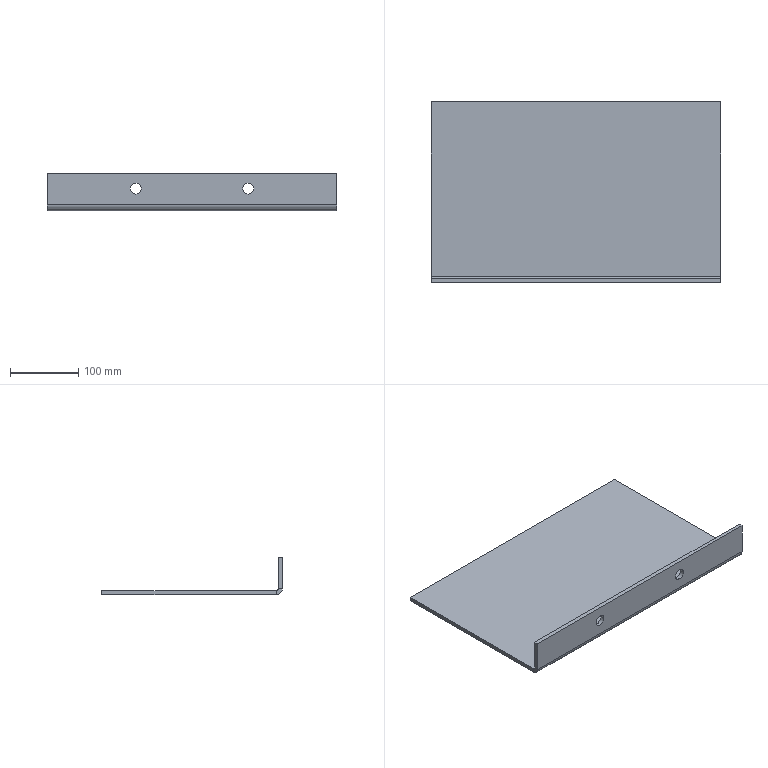Part | STEP file | Input 8 | 1 solid | 18 faces | box 425 x 265 x 55 mm | volume 792268 mm3 | plane 12 | cylinder 6 | commonest cylinder face diameters 16 x4 5 x1 17 x1
STEP:
#1=CARTESIAN_POINT('',(0.,0.,0.));
#2=DIRECTION('',(0.,0.,1.));
#3=DIRECTION('',(1.,0.,0.));
#4=AXIS2_PLACEMENT_3D('',#1,#2,#3);
#5=CARTESIAN_POINT('',(-3322.5,-300.,255.5));
#6=VERTEX_POINT('',#5);
#7=CARTESIAN_POINT('',(-3322.5,-294.,255.5));
#8=VERTEX_POINT('',#7);
#9=CARTESIAN_POINT('',(-3322.5,-300.001,255.5));
#10=DIRECTION('',(0.,1.,0.));
#11=VECTOR('',#10,1.);
#12=LINE('',#9,#11);
#13=CARTESIAN_POINT('',(-3322.5,-300.001,247.5));
#14=DIRECTION('',(0.,1.,0.));
#15=DIRECTION('',(0.,0.,1.));
#16=AXIS2_PLACEMENT_3D('',#13,#14,#15);
#17=CYLINDRICAL_SURFACE('',#16,8.);
#18=CARTESIAN_POINT('',(6.283,0.));
#19=DIRECTION('',(0.,1.));
#20=VECTOR('',#19,1.);
#21=LINE('',#18,#20);
#22=(GEOMETRIC_REPRESENTATION_CONTEXT(2)PARAMETRIC_REPRESENTATION_CONTEXT()REPRESENTATION_CONTEXT('',''));
#23=DEFINITIONAL_REPRESENTATION('',(#21),#22);
#24=PCURVE('',#17,#23);
#25=CARTESIAN_POINT('',(-3322.5,-300.001,247.5));
#26=DIRECTION('',(0.,1.,0.));
#27=DIRECTION('',(0.,0.,1.));
#28=AXIS2_PLACEMENT_3D('',#25,#26,#27);
#29=CYLINDRICAL_SURFACE('',#28,8.);
#30=CARTESIAN_POINT('',(0.,0.));
#31=DIRECTION('',(0.,1.));
#32=VECTOR('',#31,1.);
#33=LINE('',#30,#32);
#34=(GEOMETRIC_REPRESENTATION_CONTEXT(2)PARAMETRIC_REPRESENTATION_CONTEXT()REPRESENTATION_CONTEXT('',''));
#35=DEFINITIONAL_REPRESENTATION('',(#33),#34);
#36=PCURVE('',#29,#35);
#37=SURFACE_CURVE('',#12,(#24,#36),.PCURVE_S1.);
#38=EDGE_CURVE('',#6,#8,#37,.T.);
#39=ORIENTED_EDGE('',*,*,#38,.T.);
#40=CARTESIAN_POINT('',(-3322.5,-294.,239.5));
#41=VERTEX_POINT('',#40);
#42=CARTESIAN_POINT('',(-3322.5,-294.,247.5));
#43=DIRECTION('',(0.,1.,0.));
#44=DIRECTION('',(0.,0.,1.));
#45=AXIS2_PLACEMENT_3D('',#42,#43,#44);
#46=CIRCLE('',#45,8.);
#47=CARTESIAN_POINT('',(0.,6.001));
#48=DIRECTION('',(1.,0.));
#49=VECTOR('',#48,1.);
#50=LINE('',#47,#49);
#51=(GEOMETRIC_REPRESENTATION_CONTEXT(2)PARAMETRIC_REPRESENTATION_CONTEXT()REPRESENTATION_CONTEXT('',''));
#52=DEFINITIONAL_REPRESENTATION('',(#50),#51);
#53=PCURVE('',#17,#52);
#54=CARTESIAN_POINT('',(-3452.5,-294.,215.));
#55=DIRECTION('',(0.,-1.,0.));
#56=DIRECTION('',(0.,0.,-1.));
#57=AXIS2_PLACEMENT_3D('',#54,#55,#56);
#58=PLANE('',#57);
#59=CARTESIAN_POINT('',(-40.5,130.));
#60=CARTESIAN_POINT('',(-40.5,143.856));
#61=CARTESIAN_POINT('',(-28.5,136.928));
#62=CARTESIAN_POINT('',(-16.5,130.));
#63=CARTESIAN_POINT('',(-28.5,123.072));
#64=CARTESIAN_POINT('',(-40.5,116.144));
#65=CARTESIAN_POINT('',(-40.5,130.));
#66=(BOUNDED_CURVE()B_SPLINE_CURVE(2,(#59,#60,#61,#62,#63,#64,#65),.UNSPECIFIED.,.T.,.F.)B_SPLINE_CURVE_WITH_KNOTS((1,2,2,2,2,1),(-2.094,0.,2.094,4.189,6.283,8.378),.UNSPECIFIED.)CURVE()GEOMETRIC_REPRESENTATION_ITEM()RATIONAL_B_SPLINE_CURVE((1.,0.5,1.,0.5,1.,0.5,1.))REPRESENTATION_ITEM(''));
#67=(GEOMETRIC_REPRESENTATION_CONTEXT(2)PARAMETRIC_REPRESENTATION_CONTEXT()REPRESENTATION_CONTEXT('',''));
#68=DEFINITIONAL_REPRESENTATION('',(#66),#67);
#69=PCURVE('',#58,#68);
#70=SURFACE_CURVE('',#46,(#53,#69),.PCURVE_S1.);
#71=EDGE_CURVE('',#41,#8,#70,.T.);
#72=ORIENTED_EDGE('',*,*,#71,.F.);
#73=CARTESIAN_POINT('',(-3322.5,-300.,239.5));
#74=VERTEX_POINT('',#73);
#75=CARTESIAN_POINT('',(-3322.5,-300.001,239.5));
#76=DIRECTION('',(0.,1.,0.));
#77=VECTOR('',#76,1.);
#78=LINE('',#75,#77);
#79=CARTESIAN_POINT('',(3.142,0.));
#80=DIRECTION('',(0.,1.));
#81=VECTOR('',#80,1.);
#82=LINE('',#79,#81);
#83=(GEOMETRIC_REPRESENTATION_CONTEXT(2)PARAMETRIC_REPRESENTATION_CONTEXT()REPRESENTATION_CONTEXT('',''));
#84=DEFINITIONAL_REPRESENTATION('',(#82),#83);
#85=PCURVE('',#17,#84);
#86=CARTESIAN_POINT('',(3.142,0.));
#87=DIRECTION('',(0.,1.));
#88=VECTOR('',#87,1.);
#89=LINE('',#86,#88);
#90=(GEOMETRIC_REPRESENTATION_CONTEXT(2)PARAMETRIC_REPRESENTATION_CONTEXT()REPRESENTATION_CONTEXT('',''));
#91=DEFINITIONAL_REPRESENTATION('',(#89),#90);
#92=PCURVE('',#29,#91);
#93=SURFACE_CURVE('',#78,(#85,#92),.PCURVE_S1.);
#94=EDGE_CURVE('',#74,#41,#93,.T.);
#95=ORIENTED_EDGE('',*,*,#94,.F.);
#96=CARTESIAN_POINT('',(-3322.5,-300.,247.5));
#97=DIRECTION('',(0.,1.,0.));
#98=DIRECTION('',(0.,0.,-1.));
#99=AXIS2_PLACEMENT_3D('',#96,#97,#98);
#100=CIRCLE('',#99,8.);
#101=CARTESIAN_POINT('',(3.142,0.001));
#102=DIRECTION('',(1.,0.));
#103=VECTOR('',#102,1.);
#104=LINE('',#101,#103);
#105=(GEOMETRIC_REPRESENTATION_CONTEXT(2)PARAMETRIC_REPRESENTATION_CONTEXT()REPRESENTATION_CONTEXT('',''));
#106=DEFINITIONAL_REPRESENTATION('',(#104),#105);
#107=PCURVE('',#17,#106);
#108=CARTESIAN_POINT('',(-3452.5,-300.,215.));
#109=DIRECTION('',(0.,-1.,0.));
#110=DIRECTION('',(0.,0.,-1.));
#111=AXIS2_PLACEMENT_3D('',#108,#109,#110);
#112=PLANE('',#111);
#113=CARTESIAN_POINT('',(-24.5,130.));
#114=CARTESIAN_POINT('',(-24.5,116.144));
#115=CARTESIAN_POINT('',(-36.5,123.072));
#116=CARTESIAN_POINT('',(-48.5,130.));
#117=CARTESIAN_POINT('',(-36.5,136.928));
#118=CARTESIAN_POINT('',(-24.5,143.856));
#119=CARTESIAN_POINT('',(-24.5,130.));
#120=(BOUNDED_CURVE()B_SPLINE_CURVE(2,(#113,#114,#115,#116,#117,#118,#119),.UNSPECIFIED.,.T.,.F.)B_SPLINE_CURVE_WITH_KNOTS((1,2,2,2,2,1),(-2.094,0.,2.094,4.189,6.283,8.378),.UNSPECIFIED.)CURVE()GEOMETRIC_REPRESENTATION_ITEM()RATIONAL_B_SPLINE_CURVE((1.,0.5,1.,0.5,1.,0.5,1.))REPRESENTATION_ITEM(''));
#121=(GEOMETRIC_REPRESENTATION_CONTEXT(2)PARAMETRIC_REPRESENTATION_CONTEXT()REPRESENTATION_CONTEXT('',''));
#122=DEFINITIONAL_REPRESENTATION('',(#120),#121);
#123=PCURVE('',#112,#122);
#124=SURFACE_CURVE('',#100,(#107,#123),.PCURVE_S1.);
#125=EDGE_CURVE('',#74,#6,#124,.T.);
#126=ORIENTED_EDGE('',*,*,#125,.T.);
#127=EDGE_LOOP('',(#39,#72,#95,#126));
#128=FACE_BOUND('',#127,.F.);
#129=ADVANCED_FACE('',(#128),#17,.F.);
#130=CARTESIAN_POINT('',(-3157.5,-300.,255.5));
#131=VERTEX_POINT('',#130);
#132=CARTESIAN_POINT('',(-3157.5,-294.,255.5));
#133=VERTEX_POINT('',#132);
#134=CARTESIAN_POINT('',(-3157.5,-300.001,255.5));
#135=DIRECTION('',(0.,1.,0.));
#136=VECTOR('',#135,1.);
#137=LINE('',#134,#136);
#138=CARTESIAN_POINT('',(-3157.5,-300.001,247.5));
#139=DIRECTION('',(0.,1.,0.));
#140=DIRECTION('',(0.,0.,1.));
#141=AXIS2_PLACEMENT_3D('',#138,#139,#140);
#142=CYLINDRICAL_SURFACE('',#141,8.);
#143=CARTESIAN_POINT('',(6.283,0.));
#144=DIRECTION('',(0.,1.));
#145=VECTOR('',#144,1.);
#146=LINE('',#143,#145);
#147=(GEOMETRIC_REPRESENTATION_CONTEXT(2)PARAMETRIC_REPRESENTATION_CONTEXT()REPRESENTATION_CONTEXT('',''));
#148=DEFINITIONAL_REPRESENTATION('',(#146),#147);
#149=PCURVE('',#142,#148);
#150=CARTESIAN_POINT('',(-3157.5,-300.001,247.5));
#151=DIRECTION('',(0.,1.,0.));
#152=DIRECTION('',(0.,0.,1.));
#153=AXIS2_PLACEMENT_3D('',#150,#151,#152);
#154=CYLINDRICAL_SURFACE('',#153,8.);
#155=CARTESIAN_POINT('',(0.,0.));
#156=DIRECTION('',(0.,1.));
#157=VECTOR('',#156,1.);
#158=LINE('',#155,#157);
#159=(GEOMETRIC_REPRESENTATION_CONTEXT(2)PARAMETRIC_REPRESENTATION_CONTEXT()REPRESENTATION_CONTEXT('',''));
#160=DEFINITIONAL_REPRESENTATION('',(#158),#159);
#161=PCURVE('',#154,#160);
#162=SURFACE_CURVE('',#137,(#149,#161),.PCURVE_S1.);
#163=EDGE_CURVE('',#131,#133,#162,.T.);
#164=ORIENTED_EDGE('',*,*,#163,.T.);
#165=CARTESIAN_POINT('',(-3157.5,-294.,239.5));
#166=VERTEX_POINT('',#165);
#167=CARTESIAN_POINT('',(-3157.5,-294.,247.5));
#168=DIRECTION('',(0.,1.,0.));
#169=DIRECTION('',(0.,0.,1.));
#170=AXIS2_PLACEMENT_3D('',#167,#168,#169);
#171=CIRCLE('',#170,8.);
#172=CARTESIAN_POINT('',(0.,6.001));
#173=DIRECTION('',(1.,0.));
#174=VECTOR('',#173,1.);
#175=LINE('',#172,#174);
#176=(GEOMETRIC_REPRESENTATION_CONTEXT(2)PARAMETRIC_REPRESENTATION_CONTEXT()REPRESENTATION_CONTEXT('',''));
#177=DEFINITIONAL_REPRESENTATION('',(#175),#176);
#178=PCURVE('',#142,#177);
#179=CARTESIAN_POINT('',(-40.5,295.));
#180=CARTESIAN_POINT('',(-40.5,308.856));
#181=CARTESIAN_POINT('',(-28.5,301.928));
#182=CARTESIAN_POINT('',(-16.5,295.));
#183=CARTESIAN_POINT('',(-28.5,288.072));
#184=CARTESIAN_POINT('',(-40.5,281.144));
#185=CARTESIAN_POINT('',(-40.5,295.));
#186=(BOUNDED_CURVE()B_SPLINE_CURVE(2,(#179,#180,#181,#182,#183,#184,#185),.UNSPECIFIED.,.T.,.F.)B_SPLINE_CURVE_WITH_KNOTS((1,2,2,2,2,1),(-2.094,0.,2.094,4.189,6.283,8.378),.UNSPECIFIED.)CURVE()GEOMETRIC_REPRESENTATION_ITEM()RATIONAL_B_SPLINE_CURVE((1.,0.5,1.,0.5,1.,0.5,1.))REPRESENTATION_ITEM(''));
#187=(GEOMETRIC_REPRESENTATION_CONTEXT(2)PARAMETRIC_REPRESENTATION_CONTEXT()REPRESENTATION_CONTEXT('',''));
#188=DEFINITIONAL_REPRESENTATION('',(#186),#187);
#189=PCURVE('',#58,#188);
#190=SURFACE_CURVE('',#171,(#178,#189),.PCURVE_S1.);
#191=EDGE_CURVE('',#166,#133,#190,.T.);
#192=ORIENTED_EDGE('',*,*,#191,.F.);
#193=CARTESIAN_POINT('',(-3157.5,-300.,239.5));
#194=VERTEX_POINT('',#193);
#195=CARTESIAN_POINT('',(-3157.5,-300.001,239.5));
#196=DIRECTION('',(0.,1.,0.));
#197=VECTOR('',#196,1.);
#198=LINE('',#195,#197);
#199=CARTESIAN_POINT('',(3.142,0.));
#200=DIRECTION('',(0.,1.));
#201=VECTOR('',#200,1.);
#202=LINE('',#199,#201);
#203=(GEOMETRIC_REPRESENTATION_CONTEXT(2)PARAMETRIC_REPRESENTATION_CONTEXT()REPRESENTATION_CONTEXT('',''));
#204=DEFINITIONAL_REPRESENTATION('',(#202),#203);
#205=PCURVE('',#142,#204);
#206=CARTESIAN_POINT('',(3.142,0.));
#207=DIRECTION('',(0.,1.));
#208=VECTOR('',#207,1.);
#209=LINE('',#206,#208);
#210=(GEOMETRIC_REPRESENTATION_CONTEXT(2)PARAMETRIC_REPRESENTATION_CONTEXT()REPRESENTATION_CONTEXT('',''));
#211=DEFINITIONAL_REPRESENTATION('',(#209),#210);
#212=PCURVE('',#154,#211);
#213=SURFACE_CURVE('',#198,(#205,#212),.PCURVE_S1.);
#214=EDGE_CURVE('',#194,#166,#213,.T.);
#215=ORIENTED_EDGE('',*,*,#214,.F.);
#216=CARTESIAN_POINT('',(-3157.5,-300.,247.5));
#217=DIRECTION('',(0.,1.,0.));
#218=DIRECTION('',(0.,0.,-1.));
#219=AXIS2_PLACEMENT_3D('',#216,#217,#218);
#220=CIRCLE('',#219,8.);
#221=CARTESIAN_POINT('',(3.142,0.001));
#222=DIRECTION('',(1.,0.));
#223=VECTOR('',#222,1.);
#224=LINE('',#221,#223);
#225=(GEOMETRIC_REPRESENTATION_CONTEXT(2)PARAMETRIC_REPRESENTATION_CONTEXT()REPRESENTATION_CONTEXT('',''));
#226=DEFINITIONAL_REPRESENTATION('',(#224),#225);
#227=PCURVE('',#142,#226);
#228=CARTESIAN_POINT('',(-24.5,295.));
#229=CARTESIAN_POINT('',(-24.5,281.144));
#230=CARTESIAN_POINT('',(-36.5,288.072));
#231=CARTESIAN_POINT('',(-48.5,295.));
#232=CARTESIAN_POINT('',(-36.5,301.928));
#233=CARTESIAN_POINT('',(-24.5,308.856));
#234=CARTESIAN_POINT('',(-24.5,295.));
#235=(BOUNDED_CURVE()B_SPLINE_CURVE(2,(#228,#229,#230,#231,#232,#233,#234),.UNSPECIFIED.,.T.,.F.)B_SPLINE_CURVE_WITH_KNOTS((1,2,2,2,2,1),(-2.094,0.,2.094,4.189,6.283,8.378),.UNSPECIFIED.)CURVE()GEOMETRIC_REPRESENTATION_ITEM()RATIONAL_B_SPLINE_CURVE((1.,0.5,1.,0.5,1.,0.5,1.))REPRESENTATION_ITEM(''));
#236=(GEOMETRIC_REPRESENTATION_CONTEXT(2)PARAMETRIC_REPRESENTATION_CONTEXT()REPRESENTATION_CONTEXT('',''));
#237=DEFINITIONAL_REPRESENTATION('',(#235),#236);
#238=PCURVE('',#112,#237);
#239=SURFACE_CURVE('',#220,(#227,#238),.PCURVE_S1.);
#240=EDGE_CURVE('',#194,#131,#239,.T.);
#241=ORIENTED_EDGE('',*,*,#240,.T.);
#242=EDGE_LOOP('',(#164,#192,#215,#241));
#243=FACE_BOUND('',#242,.F.);
#244=ADVANCED_FACE('',(#243),#142,.F.);
#245=CARTESIAN_POINT('',(-3452.5,-291.5,215.));
#246=VERTEX_POINT('',#245);
#247=CARTESIAN_POINT('',(-3452.5,-291.5,221.));
#248=VERTEX_POINT('',#247);
#249=CARTESIAN_POINT('',(-3452.5,-291.5,215.));
#250=DIRECTION('',(0.,0.,1.));
#251=VECTOR('',#250,1.);
#252=LINE('',#249,#251);
#253=CARTESIAN_POINT('',(-3452.5,-291.5,215.));
#254=DIRECTION('',(-1.,0.,0.));
#255=DIRECTION('',(0.,0.,1.));
#256=AXIS2_PLACEMENT_3D('',#253,#254,#255);
#257=PLANE('',#256);
#258=CARTESIAN_POINT('',(0.,0.));
#259=DIRECTION('',(1.,0.));
#260=VECTOR('',#259,1.);
#261=LINE('',#258,#260);
#262=(GEOMETRIC_REPRESENTATION_CONTEXT(2)PARAMETRIC_REPRESENTATION_CONTEXT()REPRESENTATION_CONTEXT('',''));
#263=DEFINITIONAL_REPRESENTATION('',(#261),#262);
#264=PCURVE('',#257,#263);
#265=CARTESIAN_POINT('',(-3452.5,-294.,223.5));
#266=DIRECTION('',(-1.,0.,0.));
#267=DIRECTION('',(0.,0.,1.));
#268=AXIS2_PLACEMENT_3D('',#265,#266,#267);
#269=PLANE('',#268);
#270=CARTESIAN_POINT('',(-8.5,2.5));
#271=DIRECTION('',(1.,0.));
#272=VECTOR('',#271,1.);
#273=LINE('',#270,#272);
#274=(GEOMETRIC_REPRESENTATION_CONTEXT(2)PARAMETRIC_REPRESENTATION_CONTEXT()REPRESENTATION_CONTEXT('',''));
#275=DEFINITIONAL_REPRESENTATION('',(#273),#274);
#276=PCURVE('',#269,#275);
#277=SURFACE_CURVE('',#252,(#264,#276),.PCURVE_S1.);
#278=EDGE_CURVE('',#246,#248,#277,.T.);
#279=ORIENTED_EDGE('',*,*,#278,.F.);
#280=CARTESIAN_POINT('',(-3452.5,-300.,223.5));
#281=VERTEX_POINT('',#280);
#282=CARTESIAN_POINT('',(-3452.5,-291.5,223.5));
#283=DIRECTION('',(1.,0.,0.));
#284=DIRECTION('',(0.,0.,1.));
#285=AXIS2_PLACEMENT_3D('',#282,#283,#284);
#286=CIRCLE('',#285,8.5);
#287=CARTESIAN_POINT('',(17.,0.));
#288=CARTESIAN_POINT('',(17.,-14.722));
#289=CARTESIAN_POINT('',(4.25,-7.361));
#290=CARTESIAN_POINT('',(-8.5,0.));
#291=CARTESIAN_POINT('',(4.25,7.361));
#292=CARTESIAN_POINT('',(17.,14.722));
#293=CARTESIAN_POINT('',(17.,0.));
#294=(BOUNDED_CURVE()B_SPLINE_CURVE(2,(#287,#288,#289,#290,#291,#292,#293),.UNSPECIFIED.,.T.,.F.)B_SPLINE_CURVE_WITH_KNOTS((1,2,2,2,2,1),(-2.094,0.,2.094,4.189,6.283,8.378),.UNSPECIFIED.)CURVE()GEOMETRIC_REPRESENTATION_ITEM()RATIONAL_B_SPLINE_CURVE((1.,0.5,1.,0.5,1.,0.5,1.))REPRESENTATION_ITEM(''));
#295=(GEOMETRIC_REPRESENTATION_CONTEXT(2)PARAMETRIC_REPRESENTATION_CONTEXT()REPRESENTATION_CONTEXT('',''));
#296=DEFINITIONAL_REPRESENTATION('',(#294),#295);
#297=PCURVE('',#257,#296);
#298=CARTESIAN_POINT('',(-3452.5,-291.5,223.5));
#299=DIRECTION('',(1.,0.,0.));
#300=DIRECTION('',(0.,0.,-1.));
#301=AXIS2_PLACEMENT_3D('',#298,#299,#300);
#302=CYLINDRICAL_SURFACE('',#301,8.5);
#303=CARTESIAN_POINT('',(3.142,0.));
#304=DIRECTION('',(1.,0.));
#305=VECTOR('',#304,1.);
#306=LINE('',#303,#305);
#307=(GEOMETRIC_REPRESENTATION_CONTEXT(2)PARAMETRIC_REPRESENTATION_CONTEXT()REPRESENTATION_CONTEXT('',''));
#308=DEFINITIONAL_REPRESENTATION('',(#306),#307);
#309=PCURVE('',#302,#308);
#310=SURFACE_CURVE('',#286,(#297,#309),.PCURVE_S1.);
#311=EDGE_CURVE('',#281,#246,#310,.T.);
#312=ORIENTED_EDGE('',*,*,#311,.F.);
#313=CARTESIAN_POINT('',(-3452.5,-294.,223.5));
#314=VERTEX_POINT('',#313);
#315=CARTESIAN_POINT('',(-3452.5,-294.,223.5));
#316=DIRECTION('',(0.,-1.,0.));
#317=VECTOR('',#316,1.);
#318=LINE('',#315,#317);
#319=CARTESIAN_POINT('',(8.5,-2.5));
#320=DIRECTION('',(0.,-1.));
#321=VECTOR('',#320,1.);
#322=LINE('',#319,#321);
#323=(GEOMETRIC_REPRESENTATION_CONTEXT(2)PARAMETRIC_REPRESENTATION_CONTEXT()REPRESENTATION_CONTEXT('',''));
#324=DEFINITIONAL_REPRESENTATION('',(#322),#323);
#325=PCURVE('',#257,#324);
#326=CARTESIAN_POINT('',(-3452.5,-291.5,223.5));
#327=DIRECTION('',(1.,0.,0.));
#328=DIRECTION('',(0.,0.,-1.));
#329=AXIS2_PLACEMENT_3D('',#326,#327,#328);
#330=PLANE('',#329);
#331=CARTESIAN_POINT('',(0.,-2.5));
#332=DIRECTION('',(0.,-1.));
#333=VECTOR('',#332,1.);
#334=LINE('',#331,#333);
#335=(GEOMETRIC_REPRESENTATION_CONTEXT(2)PARAMETRIC_REPRESENTATION_CONTEXT()REPRESENTATION_CONTEXT('',''));
#336=DEFINITIONAL_REPRESENTATION('',(#334),#335);
#337=PCURVE('',#330,#336);
#338=SURFACE_CURVE('',#318,(#325,#337),.PCURVE_S1.);
#339=EDGE_CURVE('',#314,#281,#338,.T.);
#340=ORIENTED_EDGE('',*,*,#339,.F.);
#341=CARTESIAN_POINT('',(-3452.5,-291.5,223.5));
#342=DIRECTION('',(1.,0.,0.));
#343=DIRECTION('',(0.,0.,-1.));
#344=AXIS2_PLACEMENT_3D('',#341,#342,#343);
#345=CIRCLE('',#344,2.5);
#346=CARTESIAN_POINT('',(6.,0.));
#347=CARTESIAN_POINT('',(6.,4.33));
#348=CARTESIAN_POINT('',(9.75,2.165));
#349=CARTESIAN_POINT('',(13.5,0.));
#350=CARTESIAN_POINT('',(9.75,-2.165));
#351=CARTESIAN_POINT('',(6.,-4.33));
#352=CARTESIAN_POINT('',(6.,0.));
#353=(BOUNDED_CURVE()B_SPLINE_CURVE(2,(#346,#347,#348,#349,#350,#351,#352),.UNSPECIFIED.,.T.,.F.)B_SPLINE_CURVE_WITH_KNOTS((1,2,2,2,2,1),(-2.094,0.,2.094,4.189,6.283,8.378),.UNSPECIFIED.)CURVE()GEOMETRIC_REPRESENTATION_ITEM()RATIONAL_B_SPLINE_CURVE((1.,0.5,1.,0.5,1.,0.5,1.))REPRESENTATION_ITEM(''));
#354=(GEOMETRIC_REPRESENTATION_CONTEXT(2)PARAMETRIC_REPRESENTATION_CONTEXT()REPRESENTATION_CONTEXT('',''));
#355=DEFINITIONAL_REPRESENTATION('',(#353),#354);
#356=PCURVE('',#257,#355);
#357=CARTESIAN_POINT('',(-3452.5,-291.5,223.5));
#358=DIRECTION('',(1.,0.,0.));
#359=DIRECTION('',(0.,0.,-1.));
#360=AXIS2_PLACEMENT_3D('',#357,#358,#359);
#361=CYLINDRICAL_SURFACE('',#360,2.5);
#362=CARTESIAN_POINT('',(0.,0.));
#363=DIRECTION('',(1.,0.));
#364=VECTOR('',#363,1.);
#365=LINE('',#362,#364);
#366=(GEOMETRIC_REPRESENTATION_CONTEXT(2)PARAMETRIC_REPRESENTATION_CONTEXT()REPRESENTATION_CONTEXT('',''));
#367=DEFINITIONAL_REPRESENTATION('',(#365),#366);
#368=PCURVE('',#361,#367);
#369=SURFACE_CURVE('',#345,(#356,#368),.PCURVE_S1.);
#370=EDGE_CURVE('',#314,#248,#369,.T.);
#371=ORIENTED_EDGE('',*,*,#370,.T.);
#372=EDGE_LOOP('',(#279,#312,#340,#371));
#373=FACE_BOUND('',#372,.T.);
#374=ADVANCED_FACE('',(#373),#257,.T.);
#375=CARTESIAN_POINT('',(-3452.5,-35.,215.));
#376=VERTEX_POINT('',#375);
#377=CARTESIAN_POINT('',(-3452.5,-300.,215.));
#378=DIRECTION('',(0.,1.,0.));
#379=VECTOR('',#378,1.);
#380=LINE('',#377,#379);
#381=CARTESIAN_POINT('',(-8.5,-6.));
#382=DIRECTION('',(0.,1.));
#383=VECTOR('',#382,1.);
#384=LINE('',#381,#383);
#385=(GEOMETRIC_REPRESENTATION_CONTEXT(2)PARAMETRIC_REPRESENTATION_CONTEXT()REPRESENTATION_CONTEXT('',''));
#386=DEFINITIONAL_REPRESENTATION('',(#384),#385);
#387=PCURVE('',#269,#386);
#388=CARTESIAN_POINT('',(-3452.5,-300.,215.));
#389=DIRECTION('',(0.,0.,-1.));
#390=DIRECTION('',(-1.,0.,0.));
#391=AXIS2_PLACEMENT_3D('',#388,#389,#390);
#392=PLANE('',#391);
#393=CARTESIAN_POINT('',(0.,0.));
#394=DIRECTION('',(0.,1.));
#395=VECTOR('',#394,1.);
#396=LINE('',#393,#395);
#397=(GEOMETRIC_REPRESENTATION_CONTEXT(2)PARAMETRIC_REPRESENTATION_CONTEXT()REPRESENTATION_CONTEXT('',''));
#398=DEFINITIONAL_REPRESENTATION('',(#396),#397);
#399=PCURVE('',#392,#398);
#400=SURFACE_CURVE('',#380,(#387,#399),.PCURVE_S1.);
#401=EDGE_CURVE('',#246,#376,#400,.T.);
#402=ORIENTED_EDGE('',*,*,#401,.F.);
#403=ORIENTED_EDGE('',*,*,#278,.T.);
#404=CARTESIAN_POINT('',(-3452.5,-35.,221.));
#405=VERTEX_POINT('',#404);
#406=CARTESIAN_POINT('',(-3452.5,-300.,221.));
#407=DIRECTION('',(0.,1.,0.));
#408=VECTOR('',#407,1.);
#409=LINE('',#406,#408);
#410=CARTESIAN_POINT('',(-2.5,-6.));
#411=DIRECTION('',(0.,1.));
#412=VECTOR('',#411,1.);
#413=LINE('',#410,#412);
#414=(GEOMETRIC_REPRESENTATION_CONTEXT(2)PARAMETRIC_REPRESENTATION_CONTEXT()REPRESENTATION_CONTEXT('',''));
#415=DEFINITIONAL_REPRESENTATION('',(#413),#414);
#416=PCURVE('',#269,#415);
#417=CARTESIAN_POINT('',(-3452.5,-300.,221.));
#418=DIRECTION('',(0.,0.,-1.));
#419=DIRECTION('',(-1.,0.,0.));
#420=AXIS2_PLACEMENT_3D('',#417,#418,#419);
#421=PLANE('',#420);
#422=CARTESIAN_POINT('',(0.,0.));
#423=DIRECTION('',(0.,1.));
#424=VECTOR('',#423,1.);
#425=LINE('',#422,#424);
#426=(GEOMETRIC_REPRESENTATION_CONTEXT(2)PARAMETRIC_REPRESENTATION_CONTEXT()REPRESENTATION_CONTEXT('',''));
#427=DEFINITIONAL_REPRESENTATION('',(#425),#426);
#428=PCURVE('',#421,#427);
#429=SURFACE_CURVE('',#409,(#416,#428),.PCURVE_S1.);
#430=EDGE_CURVE('',#248,#405,#429,.T.);
#431=ORIENTED_EDGE('',*,*,#430,.T.);
#432=CARTESIAN_POINT('',(-3452.5,-35.,221.));
#433=DIRECTION('',(0.,0.,-1.));
#434=VECTOR('',#433,1.);
#435=LINE('',#432,#434);
#436=CARTESIAN_POINT('',(-2.5,259.));
#437=DIRECTION('',(-1.,0.));
#438=VECTOR('',#437,1.);
#439=LINE('',#436,#438);
#440=(GEOMETRIC_REPRESENTATION_CONTEXT(2)PARAMETRIC_REPRESENTATION_CONTEXT()REPRESENTATION_CONTEXT('',''));
#441=DEFINITIONAL_REPRESENTATION('',(#439),#440);
#442=PCURVE('',#269,#441);
#443=CARTESIAN_POINT('',(-3452.5,-35.,221.));
#444=DIRECTION('',(0.,-1.,0.));
#445=DIRECTION('',(0.,0.,-1.));
#446=AXIS2_PLACEMENT_3D('',#443,#444,#445);
#447=PLANE('',#446);
#448=CARTESIAN_POINT('',(0.,0.));
#449=DIRECTION('',(1.,0.));
#450=VECTOR('',#449,1.);
#451=LINE('',#448,#450);
#452=(GEOMETRIC_REPRESENTATION_CONTEXT(2)PARAMETRIC_REPRESENTATION_CONTEXT()REPRESENTATION_CONTEXT('',''));
#453=DEFINITIONAL_REPRESENTATION('',(#451),#452);
#454=PCURVE('',#447,#453);
#455=SURFACE_CURVE('',#435,(#442,#454),.PCURVE_S1.);
#456=EDGE_CURVE('',#405,#376,#455,.T.);
#457=ORIENTED_EDGE('',*,*,#456,.T.);
#458=EDGE_LOOP('',(#402,#403,#431,#457));
#459=FACE_BOUND('',#458,.T.);
#460=ADVANCED_FACE('',(#459),#269,.T.);
#461=CARTESIAN_POINT('',(-3027.5,-300.,223.5));
#462=VERTEX_POINT('',#461);
#463=CARTESIAN_POINT('',(-3027.5,-294.,223.5));
#464=VERTEX_POINT('',#463);
#465=CARTESIAN_POINT('',(-3027.5,-300.,223.5));
#466=DIRECTION('',(0.,1.,0.));
#467=VECTOR('',#466,1.);
#468=LINE('',#465,#467);
#469=CARTESIAN_POINT('',(-3027.5,-300.,223.5));
#470=DIRECTION('',(1.,0.,0.));
#471=DIRECTION('',(0.,0.,-1.));
#472=AXIS2_PLACEMENT_3D('',#469,#470,#471);
#473=PLANE('',#472);
#474=CARTESIAN_POINT('',(0.,0.));
#475=DIRECTION('',(0.,1.));
#476=VECTOR('',#475,1.);
#477=LINE('',#474,#476);
#478=(GEOMETRIC_REPRESENTATION_CONTEXT(2)PARAMETRIC_REPRESENTATION_CONTEXT()REPRESENTATION_CONTEXT('',''));
#479=DEFINITIONAL_REPRESENTATION('',(#477),#478);
#480=PCURVE('',#473,#479);
#481=CARTESIAN_POINT('',(-3027.5,-291.5,221.));
#482=DIRECTION('',(1.,0.,0.));
#483=DIRECTION('',(0.,0.,-1.));
#484=AXIS2_PLACEMENT_3D('',#481,#482,#483);
#485=PLANE('',#484);
#486=CARTESIAN_POINT('',(-2.5,-8.5));
#487=DIRECTION('',(0.,1.));
#488=VECTOR('',#487,1.);
#489=LINE('',#486,#488);
#490=(GEOMETRIC_REPRESENTATION_CONTEXT(2)PARAMETRIC_REPRESENTATION_CONTEXT()REPRESENTATION_CONTEXT('',''));
#491=DEFINITIONAL_REPRESENTATION('',(#489),#490);
#492=PCURVE('',#485,#491);
#493=SURFACE_CURVE('',#468,(#480,#492),.PCURVE_S1.);
#494=EDGE_CURVE('',#462,#464,#493,.T.);
#495=ORIENTED_EDGE('',*,*,#494,.F.);
#496=CARTESIAN_POINT('',(-3027.5,-291.5,215.));
#497=VERTEX_POINT('',#496);
#498=CARTESIAN_POINT('',(-3027.5,-291.5,223.5));
#499=DIRECTION('',(1.,0.,0.));
#500=DIRECTION('',(0.,0.,1.));
#501=AXIS2_PLACEMENT_3D('',#498,#499,#500);
#502=CIRCLE('',#501,8.5);
#503=CARTESIAN_POINT('',(0.,8.5));
#504=DIRECTION('',(-1.,0.));
#505=AXIS2_PLACEMENT_2D('',#503,#504);
#506=CIRCLE('',#505,8.5);
#507=(GEOMETRIC_REPRESENTATION_CONTEXT(2)PARAMETRIC_REPRESENTATION_CONTEXT()REPRESENTATION_CONTEXT('',''));
#508=DEFINITIONAL_REPRESENTATION('',(#506),#507);
#509=PCURVE('',#473,#508);
#510=CARTESIAN_POINT('',(3.142,425.));
#511=DIRECTION('',(1.,0.));
#512=VECTOR('',#511,1.);
#513=LINE('',#510,#512);
#514=(GEOMETRIC_REPRESENTATION_CONTEXT(2)PARAMETRIC_REPRESENTATION_CONTEXT()REPRESENTATION_CONTEXT('',''));
#515=DEFINITIONAL_REPRESENTATION('',(#513),#514);
#516=PCURVE('',#302,#515);
#517=SURFACE_CURVE('',#502,(#509,#516),.PCURVE_S1.);
#518=EDGE_CURVE('',#462,#497,#517,.T.);
#519=ORIENTED_EDGE('',*,*,#518,.T.);
#520=CARTESIAN_POINT('',(-3027.5,-291.5,221.));
#521=VERTEX_POINT('',#520);
#522=CARTESIAN_POINT('',(-3027.5,-291.5,221.));
#523=DIRECTION('',(0.,0.,-1.));
#524=VECTOR('',#523,1.);
#525=LINE('',#522,#524);
#526=CARTESIAN_POINT('',(2.5,8.5));
#527=DIRECTION('',(1.,0.));
#528=VECTOR('',#527,1.);
#529=LINE('',#526,#528);
#530=(GEOMETRIC_REPRESENTATION_CONTEXT(2)PARAMETRIC_REPRESENTATION_CONTEXT()REPRESENTATION_CONTEXT('',''));
#531=DEFINITIONAL_REPRESENTATION('',(#529),#530);
#532=PCURVE('',#473,#531);
#533=CARTESIAN_POINT('',(-3027.5,-291.5,223.5));
#534=DIRECTION('',(1.,0.,0.));
#535=DIRECTION('',(0.,0.,-1.));
#536=AXIS2_PLACEMENT_3D('',#533,#534,#535);
#537=PLANE('',#536);
#538=CARTESIAN_POINT('',(2.5,0.));
#539=DIRECTION('',(1.,0.));
#540=VECTOR('',#539,1.);
#541=LINE('',#538,#540);
#542=(GEOMETRIC_REPRESENTATION_CONTEXT(2)PARAMETRIC_REPRESENTATION_CONTEXT()REPRESENTATION_CONTEXT('',''));
#543=DEFINITIONAL_REPRESENTATION('',(#541),#542);
#544=PCURVE('',#537,#543);
#545=SURFACE_CURVE('',#525,(#532,#544),.PCURVE_S1.);
#546=EDGE_CURVE('',#521,#497,#545,.T.);
#547=ORIENTED_EDGE('',*,*,#546,.F.);
#548=CARTESIAN_POINT('',(-3027.5,-291.5,223.5));
#549=DIRECTION('',(1.,0.,0.));
#550=DIRECTION('',(0.,0.,-1.));
#551=AXIS2_PLACEMENT_3D('',#548,#549,#550);
#552=CIRCLE('',#551,2.5);
#553=CARTESIAN_POINT('',(0.,8.5));
#554=DIRECTION('',(1.,0.));
#555=AXIS2_PLACEMENT_2D('',#553,#554);
#556=CIRCLE('',#555,2.5);
#557=(GEOMETRIC_REPRESENTATION_CONTEXT(2)PARAMETRIC_REPRESENTATION_CONTEXT()REPRESENTATION_CONTEXT('',''));
#558=DEFINITIONAL_REPRESENTATION('',(#556),#557);
#559=PCURVE('',#473,#558);
#560=CARTESIAN_POINT('',(0.,425.));
#561=DIRECTION('',(1.,0.));
#562=VECTOR('',#561,1.);
#563=LINE('',#560,#562);
#564=(GEOMETRIC_REPRESENTATION_CONTEXT(2)PARAMETRIC_REPRESENTATION_CONTEXT()REPRESENTATION_CONTEXT('',''));
#565=DEFINITIONAL_REPRESENTATION('',(#563),#564);
#566=PCURVE('',#361,#565);
#567=SURFACE_CURVE('',#552,(#559,#566),.PCURVE_S1.);
#568=EDGE_CURVE('',#464,#521,#567,.T.);
#569=ORIENTED_EDGE('',*,*,#568,.F.);
#570=EDGE_LOOP('',(#495,#519,#547,#569));
#571=FACE_BOUND('',#570,.T.);
#572=ADVANCED_FACE('',(#571),#473,.T.);
#573=CARTESIAN_POINT('',(-3027.5,-300.,270.));
#574=VERTEX_POINT('',#573);
#575=CARTESIAN_POINT('',(-3027.5,-300.,215.));
#576=DIRECTION('',(0.,0.,-1.));
#577=VECTOR('',#576,1.);
#578=LINE('',#575,#577);
#579=CARTESIAN_POINT('',(6.,-8.5));
#580=DIRECTION('',(1.,0.));
#581=VECTOR('',#580,1.);
#582=LINE('',#579,#581);
#583=(GEOMETRIC_REPRESENTATION_CONTEXT(2)PARAMETRIC_REPRESENTATION_CONTEXT()REPRESENTATION_CONTEXT('',''));
#584=DEFINITIONAL_REPRESENTATION('',(#582),#583);
#585=PCURVE('',#485,#584);
#586=CARTESIAN_POINT('',(0.,425.));
#587=DIRECTION('',(1.,0.));
#588=VECTOR('',#587,1.);
#589=LINE('',#586,#588);
#590=(GEOMETRIC_REPRESENTATION_CONTEXT(2)PARAMETRIC_REPRESENTATION_CONTEXT()REPRESENTATION_CONTEXT('',''));
#591=DEFINITIONAL_REPRESENTATION('',(#589),#590);
#592=PCURVE('',#112,#591);
#593=SURFACE_CURVE('',#578,(#585,#592),.PCURVE_S1.);
#594=EDGE_CURVE('',#574,#462,#593,.T.);
#595=ORIENTED_EDGE('',*,*,#594,.T.);
#596=ORIENTED_EDGE('',*,*,#494,.T.);
#597=CARTESIAN_POINT('',(-3027.5,-294.,270.));
#598=VERTEX_POINT('',#597);
#599=CARTESIAN_POINT('',(-3027.5,-294.,215.));
#600=DIRECTION('',(0.,0.,-1.));
#601=VECTOR('',#600,1.);
#602=LINE('',#599,#601);
#603=CARTESIAN_POINT('',(6.,-2.5));
#604=DIRECTION('',(1.,0.));
#605=VECTOR('',#604,1.);
#606=LINE('',#603,#605);
#607=(GEOMETRIC_REPRESENTATION_CONTEXT(2)PARAMETRIC_REPRESENTATION_CONTEXT()REPRESENTATION_CONTEXT('',''));
#608=DEFINITIONAL_REPRESENTATION('',(#606),#607);
#609=PCURVE('',#485,#608);
#610=CARTESIAN_POINT('',(0.,425.));
#611=DIRECTION('',(1.,0.));
#612=VECTOR('',#611,1.);
#613=LINE('',#610,#612);
#614=(GEOMETRIC_REPRESENTATION_CONTEXT(2)PARAMETRIC_REPRESENTATION_CONTEXT()REPRESENTATION_CONTEXT('',''));
#615=DEFINITIONAL_REPRESENTATION('',(#613),#614);
#616=PCURVE('',#58,#615);
#617=SURFACE_CURVE('',#602,(#609,#616),.PCURVE_S1.);
#618=EDGE_CURVE('',#598,#464,#617,.T.);
#619=ORIENTED_EDGE('',*,*,#618,.F.);
#620=CARTESIAN_POINT('',(-3027.5,-300.,270.));
#621=DIRECTION('',(0.,1.,0.));
#622=VECTOR('',#621,1.);
#623=LINE('',#620,#622);
#624=CARTESIAN_POINT('',(-49.,-8.5));
#625=DIRECTION('',(0.,1.));
#626=VECTOR('',#625,1.);
#627=LINE('',#624,#626);
#628=(GEOMETRIC_REPRESENTATION_CONTEXT(2)PARAMETRIC_REPRESENTATION_CONTEXT()REPRESENTATION_CONTEXT('',''));
#629=DEFINITIONAL_REPRESENTATION('',(#627),#628);
#630=PCURVE('',#485,#629);
#631=CARTESIAN_POINT('',(-3452.5,-300.,270.));
#632=DIRECTION('',(0.,0.,-1.));
#633=DIRECTION('',(-1.,0.,0.));
#634=AXIS2_PLACEMENT_3D('',#631,#632,#633);
#635=PLANE('',#634);
#636=CARTESIAN_POINT('',(-425.,0.));
#637=DIRECTION('',(0.,1.));
#638=VECTOR('',#637,1.);
#639=LINE('',#636,#638);
#640=(GEOMETRIC_REPRESENTATION_CONTEXT(2)PARAMETRIC_REPRESENTATION_CONTEXT()REPRESENTATION_CONTEXT('',''));
#641=DEFINITIONAL_REPRESENTATION('',(#639),#640);
#642=PCURVE('',#635,#641);
#643=SURFACE_CURVE('',#623,(#630,#642),.PCURVE_S1.);
#644=EDGE_CURVE('',#574,#598,#643,.T.);
#645=ORIENTED_EDGE('',*,*,#644,.F.);
#646=EDGE_LOOP('',(#595,#596,#619,#645));
#647=FACE_BOUND('',#646,.T.);
#648=ADVANCED_FACE('',(#647),#485,.T.);
#649=CARTESIAN_POINT('',(-3027.5,-35.,215.));
#650=VERTEX_POINT('',#649);
#651=CARTESIAN_POINT('',(-3027.5,-300.,215.));
#652=DIRECTION('',(0.,1.,0.));
#653=VECTOR('',#652,1.);
#654=LINE('',#651,#653);
#655=CARTESIAN_POINT('',(-425.,0.));
#656=DIRECTION('',(0.,1.));
#657=VECTOR('',#656,1.);
#658=LINE('',#655,#657);
#659=(GEOMETRIC_REPRESENTATION_CONTEXT(2)PARAMETRIC_REPRESENTATION_CONTEXT()REPRESENTATION_CONTEXT('',''));
#660=DEFINITIONAL_REPRESENTATION('',(#658),#659);
#661=PCURVE('',#392,#660);
#662=CARTESIAN_POINT('',(8.5,-8.5));
#663=DIRECTION('',(0.,1.));
#664=VECTOR('',#663,1.);
#665=LINE('',#662,#664);
#666=(GEOMETRIC_REPRESENTATION_CONTEXT(2)PARAMETRIC_REPRESENTATION_CONTEXT()REPRESENTATION_CONTEXT('',''));
#667=DEFINITIONAL_REPRESENTATION('',(#665),#666);
#668=PCURVE('',#537,#667);
#669=SURFACE_CURVE('',#654,(#661,#668),.PCURVE_S1.);
#670=EDGE_CURVE('',#497,#650,#669,.T.);
#671=ORIENTED_EDGE('',*,*,#670,.F.);
#672=CARTESIAN_POINT('',(-3452.5,-291.5,215.));
#673=DIRECTION('',(1.,0.,0.));
#674=VECTOR('',#673,1.);
#675=LINE('',#672,#674);
#676=CARTESIAN_POINT('',(0.,8.5));
#677=DIRECTION('',(-1.,0.));
#678=VECTOR('',#677,1.);
#679=LINE('',#676,#678);
#680=(GEOMETRIC_REPRESENTATION_CONTEXT(2)PARAMETRIC_REPRESENTATION_CONTEXT()REPRESENTATION_CONTEXT('',''));
#681=DEFINITIONAL_REPRESENTATION('',(#679),#680);
#682=PCURVE('',#392,#681);
#683=CARTESIAN_POINT('',(6.283,0.));
#684=DIRECTION('',(0.,1.));
#685=VECTOR('',#684,1.);
#686=LINE('',#683,#685);
#687=(GEOMETRIC_REPRESENTATION_CONTEXT(2)PARAMETRIC_REPRESENTATION_CONTEXT()REPRESENTATION_CONTEXT('',''));
#688=DEFINITIONAL_REPRESENTATION('',(#686),#687);
#689=PCURVE('',#302,#688);
#690=SURFACE_CURVE('',#675,(#682,#689),.PCURVE_S1.);
#691=EDGE_CURVE('',#246,#497,#690,.T.);
#692=ORIENTED_EDGE('',*,*,#691,.F.);
#693=ORIENTED_EDGE('',*,*,#401,.T.);
#694=CARTESIAN_POINT('',(-3452.5,-35.,215.));
#695=DIRECTION('',(1.,0.,0.));
#696=VECTOR('',#695,1.);
#697=LINE('',#694,#696);
#698=CARTESIAN_POINT('',(0.,265.));
#699=DIRECTION('',(-1.,0.));
#700=VECTOR('',#699,1.);
#701=LINE('',#698,#700);
#702=(GEOMETRIC_REPRESENTATION_CONTEXT(2)PARAMETRIC_REPRESENTATION_CONTEXT()REPRESENTATION_CONTEXT('',''));
#703=DEFINITIONAL_REPRESENTATION('',(#701),#702);
#704=PCURVE('',#392,#703);
#705=CARTESIAN_POINT('',(6.,0.));
#706=DIRECTION('',(0.,1.));
#707=VECTOR('',#706,1.);
#708=LINE('',#705,#707);
#709=(GEOMETRIC_REPRESENTATION_CONTEXT(2)PARAMETRIC_REPRESENTATION_CONTEXT()REPRESENTATION_CONTEXT('',''));
#710=DEFINITIONAL_REPRESENTATION('',(#708),#709);
#711=PCURVE('',#447,#710);
#712=SURFACE_CURVE('',#697,(#704,#711),.PCURVE_S1.);
#713=EDGE_CURVE('',#376,#650,#712,.T.);
#714=ORIENTED_EDGE('',*,*,#713,.T.);
#715=EDGE_LOOP('',(#671,#692,#693,#714));
#716=FACE_BOUND('',#715,.T.);
#717=ADVANCED_FACE('',(#716),#392,.T.);
#718=ORIENTED_EDGE('',*,*,#518,.F.);
#719=CARTESIAN_POINT('',(-3452.5,-300.,223.5));
#720=DIRECTION('',(1.,0.,0.));
#721=VECTOR('',#720,1.);
#722=LINE('',#719,#721);
#723=CARTESIAN_POINT('',(4.712,0.));
#724=DIRECTION('',(0.,1.));
#725=VECTOR('',#724,1.);
#726=LINE('',#723,#725);
#727=(GEOMETRIC_REPRESENTATION_CONTEXT(2)PARAMETRIC_REPRESENTATION_CONTEXT()REPRESENTATION_CONTEXT('',''));
#728=DEFINITIONAL_REPRESENTATION('',(#726),#727);
#729=PCURVE('',#302,#728);
#730=CARTESIAN_POINT('',(-8.5,0.));
#731=DIRECTION('',(0.,1.));
#732=VECTOR('',#731,1.);
#733=LINE('',#730,#732);
#734=(GEOMETRIC_REPRESENTATION_CONTEXT(2)PARAMETRIC_REPRESENTATION_CONTEXT()REPRESENTATION_CONTEXT('',''));
#735=DEFINITIONAL_REPRESENTATION('',(#733),#734);
#736=PCURVE('',#112,#735);
#737=SURFACE_CURVE('',#722,(#729,#736),.PCURVE_S1.);
#738=EDGE_CURVE('',#281,#462,#737,.T.);
#739=ORIENTED_EDGE('',*,*,#738,.F.);
#740=ORIENTED_EDGE('',*,*,#311,.T.);
#741=ORIENTED_EDGE('',*,*,#691,.T.);
#742=EDGE_LOOP('',(#718,#739,#740,#741));
#743=FACE_BOUND('',#742,.T.);
#744=ADVANCED_FACE('',(#743),#302,.T.);
#745=CARTESIAN_POINT('',(-3322.5,-300.,247.5));
#746=DIRECTION('',(0.,1.,0.));
#747=DIRECTION('',(0.,0.,-1.));
#748=AXIS2_PLACEMENT_3D('',#745,#746,#747);
#749=CIRCLE('',#748,8.);
#750=CARTESIAN_POINT('',(-24.5,130.));
#751=CARTESIAN_POINT('',(-24.5,116.144));
#752=CARTESIAN_POINT('',(-36.5,123.072));
#753=CARTESIAN_POINT('',(-48.5,130.));
#754=CARTESIAN_POINT('',(-36.5,136.928));
#755=CARTESIAN_POINT('',(-24.5,143.856));
#756=CARTESIAN_POINT('',(-24.5,130.));
#757=(BOUNDED_CURVE()B_SPLINE_CURVE(2,(#750,#751,#752,#753,#754,#755,#756),.UNSPECIFIED.,.T.,.F.)B_SPLINE_CURVE_WITH_KNOTS((1,2,2,2,2,1),(-2.094,0.,2.094,4.189,6.283,8.378),.UNSPECIFIED.)CURVE()GEOMETRIC_REPRESENTATION_ITEM()RATIONAL_B_SPLINE_CURVE((1.,0.5,1.,0.5,1.,0.5,1.))REPRESENTATION_ITEM(''));
#758=(GEOMETRIC_REPRESENTATION_CONTEXT(2)PARAMETRIC_REPRESENTATION_CONTEXT()REPRESENTATION_CONTEXT('',''));
#759=DEFINITIONAL_REPRESENTATION('',(#757),#758);
#760=PCURVE('',#112,#759);
#761=CARTESIAN_POINT('',(-3.142,0.001));
#762=DIRECTION('',(1.,0.));
#763=VECTOR('',#762,1.);
#764=LINE('',#761,#763);
#765=(GEOMETRIC_REPRESENTATION_CONTEXT(2)PARAMETRIC_REPRESENTATION_CONTEXT()REPRESENTATION_CONTEXT('',''));
#766=DEFINITIONAL_REPRESENTATION('',(#764),#765);
#767=PCURVE('',#29,#766);
#768=SURFACE_CURVE('',#749,(#760,#767),.PCURVE_S1.);
#769=EDGE_CURVE('',#6,#74,#768,.T.);
#770=ORIENTED_EDGE('',*,*,#769,.T.);
#771=ORIENTED_EDGE('',*,*,#125,.T.);
#772=EDGE_LOOP('',(#770,#771));
#773=FACE_BOUND('',#772,.T.);
#774=CARTESIAN_POINT('',(-3157.5,-300.,247.5));
#775=DIRECTION('',(0.,1.,0.));
#776=DIRECTION('',(0.,0.,-1.));
#777=AXIS2_PLACEMENT_3D('',#774,#775,#776);
#778=CIRCLE('',#777,8.);
#779=CARTESIAN_POINT('',(-24.5,295.));
#780=CARTESIAN_POINT('',(-24.5,281.144));
#781=CARTESIAN_POINT('',(-36.5,288.072));
#782=CARTESIAN_POINT('',(-48.5,295.));
#783=CARTESIAN_POINT('',(-36.5,301.928));
#784=CARTESIAN_POINT('',(-24.5,308.856));
#785=CARTESIAN_POINT('',(-24.5,295.));
#786=(BOUNDED_CURVE()B_SPLINE_CURVE(2,(#779,#780,#781,#782,#783,#784,#785),.UNSPECIFIED.,.T.,.F.)B_SPLINE_CURVE_WITH_KNOTS((1,2,2,2,2,1),(-2.094,0.,2.094,4.189,6.283,8.378),.UNSPECIFIED.)CURVE()GEOMETRIC_REPRESENTATION_ITEM()RATIONAL_B_SPLINE_CURVE((1.,0.5,1.,0.5,1.,0.5,1.))REPRESENTATION_ITEM(''));
#787=(GEOMETRIC_REPRESENTATION_CONTEXT(2)PARAMETRIC_REPRESENTATION_CONTEXT()REPRESENTATION_CONTEXT('',''));
#788=DEFINITIONAL_REPRESENTATION('',(#786),#787);
#789=PCURVE('',#112,#788);
#790=CARTESIAN_POINT('',(-3.142,0.001));
#791=DIRECTION('',(1.,0.));
#792=VECTOR('',#791,1.);
#793=LINE('',#790,#792);
#794=(GEOMETRIC_REPRESENTATION_CONTEXT(2)PARAMETRIC_REPRESENTATION_CONTEXT()REPRESENTATION_CONTEXT('',''));
#795=DEFINITIONAL_REPRESENTATION('',(#793),#794);
#796=PCURVE('',#154,#795);
#797=SURFACE_CURVE('',#778,(#789,#796),.PCURVE_S1.);
#798=EDGE_CURVE('',#131,#194,#797,.T.);
#799=ORIENTED_EDGE('',*,*,#798,.T.);
#800=ORIENTED_EDGE('',*,*,#240,.T.);
#801=EDGE_LOOP('',(#799,#800));
#802=FACE_BOUND('',#801,.T.);
#803=ORIENTED_EDGE('',*,*,#594,.F.);
#804=CARTESIAN_POINT('',(-3452.5,-300.,270.));
#805=VERTEX_POINT('',#804);
#806=CARTESIAN_POINT('',(-3452.5,-300.,270.));
#807=DIRECTION('',(1.,0.,0.));
#808=VECTOR('',#807,1.);
#809=LINE('',#806,#808);
#810=CARTESIAN_POINT('',(-55.,0.));
#811=DIRECTION('',(0.,1.));
#812=VECTOR('',#811,1.);
#813=LINE('',#810,#812);
#814=(GEOMETRIC_REPRESENTATION_CONTEXT(2)PARAMETRIC_REPRESENTATION_CONTEXT()REPRESENTATION_CONTEXT('',''));
#815=DEFINITIONAL_REPRESENTATION('',(#813),#814);
#816=PCURVE('',#112,#815);
#817=CARTESIAN_POINT('',(0.,0.));
#818=DIRECTION('',(-1.,0.));
#819=VECTOR('',#818,1.);
#820=LINE('',#817,#819);
#821=(GEOMETRIC_REPRESENTATION_CONTEXT(2)PARAMETRIC_REPRESENTATION_CONTEXT()REPRESENTATION_CONTEXT('',''));
#822=DEFINITIONAL_REPRESENTATION('',(#820),#821);
#823=PCURVE('',#635,#822);
#824=SURFACE_CURVE('',#809,(#816,#823),.PCURVE_S1.);
#825=EDGE_CURVE('',#805,#574,#824,.T.);
#826=ORIENTED_EDGE('',*,*,#825,.F.);
#827=CARTESIAN_POINT('',(-3452.5,-300.,215.));
#828=DIRECTION('',(0.,0.,-1.));
#829=VECTOR('',#828,1.);
#830=LINE('',#827,#829);
#831=CARTESIAN_POINT('',(0.,0.));
#832=DIRECTION('',(1.,0.));
#833=VECTOR('',#832,1.);
#834=LINE('',#831,#833);
#835=(GEOMETRIC_REPRESENTATION_CONTEXT(2)PARAMETRIC_REPRESENTATION_CONTEXT()REPRESENTATION_CONTEXT('',''));
#836=DEFINITIONAL_REPRESENTATION('',(#834),#835);
#837=PCURVE('',#112,#836);
#838=CARTESIAN_POINT('',(8.5,-8.5));
#839=DIRECTION('',(1.,0.));
#840=VECTOR('',#839,1.);
#841=LINE('',#838,#840);
#842=(GEOMETRIC_REPRESENTATION_CONTEXT(2)PARAMETRIC_REPRESENTATION_CONTEXT()REPRESENTATION_CONTEXT('',''));
#843=DEFINITIONAL_REPRESENTATION('',(#841),#842);
#844=PCURVE('',#330,#843);
#845=SURFACE_CURVE('',#830,(#837,#844),.PCURVE_S1.);
#846=EDGE_CURVE('',#805,#281,#845,.T.);
#847=ORIENTED_EDGE('',*,*,#846,.T.);
#848=ORIENTED_EDGE('',*,*,#738,.T.);
#849=EDGE_LOOP('',(#803,#826,#847,#848));
#850=FACE_BOUND('',#849,.T.);
#851=ADVANCED_FACE('',(#773,#802,#850),#112,.T.);
#852=ORIENTED_EDGE('',*,*,#644,.T.);
#853=CARTESIAN_POINT('',(-3452.5,-294.,270.));
#854=VERTEX_POINT('',#853);
#855=CARTESIAN_POINT('',(-3452.5,-294.,270.));
#856=DIRECTION('',(1.,0.,0.));
#857=VECTOR('',#856,1.);
#858=LINE('',#855,#857);
#859=CARTESIAN_POINT('',(0.,6.));
#860=DIRECTION('',(-1.,0.));
#861=VECTOR('',#860,1.);
#862=LINE('',#859,#861);
#863=(GEOMETRIC_REPRESENTATION_CONTEXT(2)PARAMETRIC_REPRESENTATION_CONTEXT()REPRESENTATION_CONTEXT('',''));
#864=DEFINITIONAL_REPRESENTATION('',(#862),#863);
#865=PCURVE('',#635,#864);
#866=CARTESIAN_POINT('',(-55.,0.));
#867=DIRECTION('',(0.,1.));
#868=VECTOR('',#867,1.);
#869=LINE('',#866,#868);
#870=(GEOMETRIC_REPRESENTATION_CONTEXT(2)PARAMETRIC_REPRESENTATION_CONTEXT()REPRESENTATION_CONTEXT('',''));
#871=DEFINITIONAL_REPRESENTATION('',(#869),#870);
#872=PCURVE('',#58,#871);
#873=SURFACE_CURVE('',#858,(#865,#872),.PCURVE_S1.);
#874=EDGE_CURVE('',#854,#598,#873,.T.);
#875=ORIENTED_EDGE('',*,*,#874,.F.);
#876=CARTESIAN_POINT('',(-3452.5,-300.,270.));
#877=DIRECTION('',(0.,1.,0.));
#878=VECTOR('',#877,1.);
#879=LINE('',#876,#878);
#880=CARTESIAN_POINT('',(0.,0.));
#881=DIRECTION('',(0.,1.));
#882=VECTOR('',#881,1.);
#883=LINE('',#880,#882);
#884=(GEOMETRIC_REPRESENTATION_CONTEXT(2)PARAMETRIC_REPRESENTATION_CONTEXT()REPRESENTATION_CONTEXT('',''));
#885=DEFINITIONAL_REPRESENTATION('',(#883),#884);
#886=PCURVE('',#635,#885);
#887=CARTESIAN_POINT('',(-46.5,-8.5));
#888=DIRECTION('',(0.,1.));
#889=VECTOR('',#888,1.);
#890=LINE('',#887,#889);
#891=(GEOMETRIC_REPRESENTATION_CONTEXT(2)PARAMETRIC_REPRESENTATION_CONTEXT()REPRESENTATION_CONTEXT('',''));
#892=DEFINITIONAL_REPRESENTATION('',(#890),#891);
#893=PCURVE('',#330,#892);
#894=SURFACE_CURVE('',#879,(#886,#893),.PCURVE_S1.);
#895=EDGE_CURVE('',#805,#854,#894,.T.);
#896=ORIENTED_EDGE('',*,*,#895,.F.);
#897=ORIENTED_EDGE('',*,*,#825,.T.);
#898=EDGE_LOOP('',(#852,#875,#896,#897));
#899=FACE_BOUND('',#898,.T.);
#900=ADVANCED_FACE('',(#899),#635,.F.);
#901=CARTESIAN_POINT('',(-3322.5,-294.,247.5));
#902=DIRECTION('',(0.,1.,0.));
#903=DIRECTION('',(0.,0.,1.));
#904=AXIS2_PLACEMENT_3D('',#901,#902,#903);
#905=CIRCLE('',#904,8.);
#906=CARTESIAN_POINT('',(-40.5,130.));
#907=CARTESIAN_POINT('',(-40.5,143.856));
#908=CARTESIAN_POINT('',(-28.5,136.928));
#909=CARTESIAN_POINT('',(-16.5,130.));
#910=CARTESIAN_POINT('',(-28.5,123.072));
#911=CARTESIAN_POINT('',(-40.5,116.144));
#912=CARTESIAN_POINT('',(-40.5,130.));
#913=(BOUNDED_CURVE()B_SPLINE_CURVE(2,(#906,#907,#908,#909,#910,#911,#912),.UNSPECIFIED.,.T.,.F.)B_SPLINE_CURVE_WITH_KNOTS((1,2,2,2,2,1),(-2.094,0.,2.094,4.189,6.283,8.378),.UNSPECIFIED.)CURVE()GEOMETRIC_REPRESENTATION_ITEM()RATIONAL_B_SPLINE_CURVE((1.,0.5,1.,0.5,1.,0.5,1.))REPRESENTATION_ITEM(''));
#914=(GEOMETRIC_REPRESENTATION_CONTEXT(2)PARAMETRIC_REPRESENTATION_CONTEXT()REPRESENTATION_CONTEXT('',''));
#915=DEFINITIONAL_REPRESENTATION('',(#913),#914);
#916=PCURVE('',#58,#915);
#917=CARTESIAN_POINT('',(0.,6.001));
#918=DIRECTION('',(1.,0.));
#919=VECTOR('',#918,1.);
#920=LINE('',#917,#919);
#921=(GEOMETRIC_REPRESENTATION_CONTEXT(2)PARAMETRIC_REPRESENTATION_CONTEXT()REPRESENTATION_CONTEXT('',''));
#922=DEFINITIONAL_REPRESENTATION('',(#920),#921);
#923=PCURVE('',#29,#922);
#924=SURFACE_CURVE('',#905,(#916,#923),.PCURVE_S1.);
#925=EDGE_CURVE('',#8,#41,#924,.T.);
#926=ORIENTED_EDGE('',*,*,#925,.F.);
#927=ORIENTED_EDGE('',*,*,#71,.F.);
#928=EDGE_LOOP('',(#926,#927));
#929=FACE_BOUND('',#928,.T.);
#930=CARTESIAN_POINT('',(-3157.5,-294.,247.5));
#931=DIRECTION('',(0.,1.,0.));
#932=DIRECTION('',(0.,0.,1.));
#933=AXIS2_PLACEMENT_3D('',#930,#931,#932);
#934=CIRCLE('',#933,8.);
#935=CARTESIAN_POINT('',(-40.5,295.));
#936=CARTESIAN_POINT('',(-40.5,308.856));
#937=CARTESIAN_POINT('',(-28.5,301.928));
#938=CARTESIAN_POINT('',(-16.5,295.));
#939=CARTESIAN_POINT('',(-28.5,288.072));
#940=CARTESIAN_POINT('',(-40.5,281.144));
#941=CARTESIAN_POINT('',(-40.5,295.));
#942=(BOUNDED_CURVE()B_SPLINE_CURVE(2,(#935,#936,#937,#938,#939,#940,#941),.UNSPECIFIED.,.T.,.F.)B_SPLINE_CURVE_WITH_KNOTS((1,2,2,2,2,1),(-2.094,0.,2.094,4.189,6.283,8.378),.UNSPECIFIED.)CURVE()GEOMETRIC_REPRESENTATION_ITEM()RATIONAL_B_SPLINE_CURVE((1.,0.5,1.,0.5,1.,0.5,1.))REPRESENTATION_ITEM(''));
#943=(GEOMETRIC_REPRESENTATION_CONTEXT(2)PARAMETRIC_REPRESENTATION_CONTEXT()REPRESENTATION_CONTEXT('',''));
#944=DEFINITIONAL_REPRESENTATION('',(#942),#943);
#945=PCURVE('',#58,#944);
#946=CARTESIAN_POINT('',(0.,6.001));
#947=DIRECTION('',(1.,0.));
#948=VECTOR('',#947,1.);
#949=LINE('',#946,#948);
#950=(GEOMETRIC_REPRESENTATION_CONTEXT(2)PARAMETRIC_REPRESENTATION_CONTEXT()REPRESENTATION_CONTEXT('',''));
#951=DEFINITIONAL_REPRESENTATION('',(#949),#950);
#952=PCURVE('',#154,#951);
#953=SURFACE_CURVE('',#934,(#945,#952),.PCURVE_S1.);
#954=EDGE_CURVE('',#133,#166,#953,.T.);
#955=ORIENTED_EDGE('',*,*,#954,.F.);
#956=ORIENTED_EDGE('',*,*,#191,.F.);
#957=EDGE_LOOP('',(#955,#956));
#958=FACE_BOUND('',#957,.T.);
#959=ORIENTED_EDGE('',*,*,#618,.T.);
#960=CARTESIAN_POINT('',(-3452.5,-294.,223.5));
#961=DIRECTION('',(1.,0.,0.));
#962=VECTOR('',#961,1.);
#963=LINE('',#960,#962);
#964=CARTESIAN_POINT('',(-8.5,0.));
#965=DIRECTION('',(0.,1.));
#966=VECTOR('',#965,1.);
#967=LINE('',#964,#966);
#968=(GEOMETRIC_REPRESENTATION_CONTEXT(2)PARAMETRIC_REPRESENTATION_CONTEXT()REPRESENTATION_CONTEXT('',''));
#969=DEFINITIONAL_REPRESENTATION('',(#967),#968);
#970=PCURVE('',#58,#969);
#971=CARTESIAN_POINT('',(4.712,0.));
#972=DIRECTION('',(0.,1.));
#973=VECTOR('',#972,1.);
#974=LINE('',#971,#973);
#975=(GEOMETRIC_REPRESENTATION_CONTEXT(2)PARAMETRIC_REPRESENTATION_CONTEXT()REPRESENTATION_CONTEXT('',''));
#976=DEFINITIONAL_REPRESENTATION('',(#974),#975);
#977=PCURVE('',#361,#976);
#978=SURFACE_CURVE('',#963,(#970,#977),.PCURVE_S1.);
#979=EDGE_CURVE('',#314,#464,#978,.T.);
#980=ORIENTED_EDGE('',*,*,#979,.F.);
#981=CARTESIAN_POINT('',(-3452.5,-294.,215.));
#982=DIRECTION('',(0.,0.,-1.));
#983=VECTOR('',#982,1.);
#984=LINE('',#981,#983);
#985=CARTESIAN_POINT('',(0.,0.));
#986=DIRECTION('',(1.,0.));
#987=VECTOR('',#986,1.);
#988=LINE('',#985,#987);
#989=(GEOMETRIC_REPRESENTATION_CONTEXT(2)PARAMETRIC_REPRESENTATION_CONTEXT()REPRESENTATION_CONTEXT('',''));
#990=DEFINITIONAL_REPRESENTATION('',(#988),#989);
#991=PCURVE('',#58,#990);
#992=CARTESIAN_POINT('',(8.5,-2.5));
#993=DIRECTION('',(1.,0.));
#994=VECTOR('',#993,1.);
#995=LINE('',#992,#994);
#996=(GEOMETRIC_REPRESENTATION_CONTEXT(2)PARAMETRIC_REPRESENTATION_CONTEXT()REPRESENTATION_CONTEXT('',''));
#997=DEFINITIONAL_REPRESENTATION('',(#995),#996);
#998=PCURVE('',#330,#997);
#999=SURFACE_CURVE('',#984,(#991,#998),.PCURVE_S1.);
#1000=EDGE_CURVE('',#854,#314,#999,.T.);
#1001=ORIENTED_EDGE('',*,*,#1000,.F.);
#1002=ORIENTED_EDGE('',*,*,#874,.T.);
#1003=EDGE_LOOP('',(#959,#980,#1001,#1002));
#1004=FACE_BOUND('',#1003,.T.);
#1005=ADVANCED_FACE('',(#929,#958,#1004),#58,.F.);
#1006=ORIENTED_EDGE('',*,*,#979,.F.);
#1007=ORIENTED_EDGE('',*,*,#370,.T.);
#1008=CARTESIAN_POINT('',(-3452.5,-291.5,221.));
#1009=DIRECTION('',(1.,0.,0.));
#1010=VECTOR('',#1009,1.);
#1011=LINE('',#1008,#1010);
#1012=CARTESIAN_POINT('',(6.283,0.));
#1013=DIRECTION('',(0.,1.));
#1014=VECTOR('',#1013,1.);
#1015=LINE('',#1012,#1014);
#1016=(GEOMETRIC_REPRESENTATION_CONTEXT(2)PARAMETRIC_REPRESENTATION_CONTEXT()REPRESENTATION_CONTEXT('',''));
#1017=DEFINITIONAL_REPRESENTATION('',(#1015),#1016);
#1018=PCURVE('',#361,#1017);
#1019=CARTESIAN_POINT('',(0.,8.5));
#1020=DIRECTION('',(-1.,0.));
#1021=VECTOR('',#1020,1.);
#1022=LINE('',#1019,#1021);
#1023=(GEOMETRIC_REPRESENTATION_CONTEXT(2)PARAMETRIC_REPRESENTATION_CONTEXT()REPRESENTATION_CONTEXT('',''));
#1024=DEFINITIONAL_REPRESENTATION('',(#1022),#1023);
#1025=PCURVE('',#421,#1024);
#1026=SURFACE_CURVE('',#1011,(#1018,#1025),.PCURVE_S1.);
#1027=EDGE_CURVE('',#248,#521,#1026,.T.);
#1028=ORIENTED_EDGE('',*,*,#1027,.T.);
#1029=ORIENTED_EDGE('',*,*,#568,.F.);
#1030=EDGE_LOOP('',(#1006,#1007,#1028,#1029));
#1031=FACE_BOUND('',#1030,.F.);
#1032=ADVANCED_FACE('',(#1031),#361,.F.);
#1033=CARTESIAN_POINT('',(-3027.5,-35.,221.));
#1034=VERTEX_POINT('',#1033);
#1035=CARTESIAN_POINT('',(-3027.5,-300.,221.));
#1036=DIRECTION('',(0.,1.,0.));
#1037=VECTOR('',#1036,1.);
#1038=LINE('',#1035,#1037);
#1039=CARTESIAN_POINT('',(-425.,0.));
#1040=DIRECTION('',(0.,1.));
#1041=VECTOR('',#1040,1.);
#1042=LINE('',#1039,#1041);
#1043=(GEOMETRIC_REPRESENTATION_CONTEXT(2)PARAMETRIC_REPRESENTATION_CONTEXT()REPRESENTATION_CONTEXT('',''));
#1044=DEFINITIONAL_REPRESENTATION('',(#1042),#1043);
#1045=PCURVE('',#421,#1044);
#1046=CARTESIAN_POINT('',(2.5,-8.5));
#1047=DIRECTION('',(0.,1.));
#1048=VECTOR('',#1047,1.);
#1049=LINE('',#1046,#1048);
#1050=(GEOMETRIC_REPRESENTATION_CONTEXT(2)PARAMETRIC_REPRESENTATION_CONTEXT()REPRESENTATION_CONTEXT('',''));
#1051=DEFINITIONAL_REPRESENTATION('',(#1049),#1050);
#1052=PCURVE('',#537,#1051);
#1053=SURFACE_CURVE('',#1038,(#1045,#1052),.PCURVE_S1.);
#1054=EDGE_CURVE('',#521,#1034,#1053,.T.);
#1055=ORIENTED_EDGE('',*,*,#1054,.T.);
#1056=CARTESIAN_POINT('',(-3452.5,-35.,221.));
#1057=DIRECTION('',(1.,0.,0.));
#1058=VECTOR('',#1057,1.);
#1059=LINE('',#1056,#1058);
#1060=CARTESIAN_POINT('',(0.,265.));
#1061=DIRECTION('',(-1.,0.));
#1062=VECTOR('',#1061,1.);
#1063=LINE('',#1060,#1062);
#1064=(GEOMETRIC_REPRESENTATION_CONTEXT(2)PARAMETRIC_REPRESENTATION_CONTEXT()REPRESENTATION_CONTEXT('',''));
#1065=DEFINITIONAL_REPRESENTATION('',(#1063),#1064);
#1066=PCURVE('',#421,#1065);
#1067=CARTESIAN_POINT('',(0.,0.));
#1068=DIRECTION('',(0.,1.));
#1069=VECTOR('',#1068,1.);
#1070=LINE('',#1067,#1069);
#1071=(GEOMETRIC_REPRESENTATION_CONTEXT(2)PARAMETRIC_REPRESENTATION_CONTEXT()REPRESENTATION_CONTEXT('',''));
#1072=DEFINITIONAL_REPRESENTATION('',(#1070),#1071);
#1073=PCURVE('',#447,#1072);
#1074=SURFACE_CURVE('',#1059,(#1066,#1073),.PCURVE_S1.);
#1075=EDGE_CURVE('',#405,#1034,#1074,.T.);
#1076=ORIENTED_EDGE('',*,*,#1075,.F.);
#1077=ORIENTED_EDGE('',*,*,#430,.F.);
#1078=ORIENTED_EDGE('',*,*,#1027,.T.);
#1079=EDGE_LOOP('',(#1055,#1076,#1077,#1078));
#1080=FACE_BOUND('',#1079,.T.);
#1081=ADVANCED_FACE('',(#1080),#421,.F.);
#1082=CARTESIAN_POINT('',(-3027.5,-35.,221.));
#1083=DIRECTION('',(0.,0.,-1.));
#1084=VECTOR('',#1083,1.);
#1085=LINE('',#1082,#1084);
#1086=CARTESIAN_POINT('',(0.,425.));
#1087=DIRECTION('',(1.,0.));
#1088=VECTOR('',#1087,1.);
#1089=LINE('',#1086,#1088);
#1090=(GEOMETRIC_REPRESENTATION_CONTEXT(2)PARAMETRIC_REPRESENTATION_CONTEXT()REPRESENTATION_CONTEXT('',''));
#1091=DEFINITIONAL_REPRESENTATION('',(#1089),#1090);
#1092=PCURVE('',#447,#1091);
#1093=CARTESIAN_POINT('',(2.5,256.5));
#1094=DIRECTION('',(1.,0.));
#1095=VECTOR('',#1094,1.);
#1096=LINE('',#1093,#1095);
#1097=(GEOMETRIC_REPRESENTATION_CONTEXT(2)PARAMETRIC_REPRESENTATION_CONTEXT()REPRESENTATION_CONTEXT('',''));
#1098=DEFINITIONAL_REPRESENTATION('',(#1096),#1097);
#1099=PCURVE('',#537,#1098);
#1100=SURFACE_CURVE('',#1085,(#1092,#1099),.PCURVE_S1.);
#1101=EDGE_CURVE('',#1034,#650,#1100,.T.);
#1102=ORIENTED_EDGE('',*,*,#1101,.T.);
#1103=ORIENTED_EDGE('',*,*,#713,.F.);
#1104=ORIENTED_EDGE('',*,*,#456,.F.);
#1105=ORIENTED_EDGE('',*,*,#1075,.T.);
#1106=EDGE_LOOP('',(#1102,#1103,#1104,#1105));
#1107=FACE_BOUND('',#1106,.T.);
#1108=ADVANCED_FACE('',(#1107),#447,.F.);
#1109=ORIENTED_EDGE('',*,*,#1000,.T.);
#1110=ORIENTED_EDGE('',*,*,#339,.T.);
#1111=ORIENTED_EDGE('',*,*,#846,.F.);
#1112=ORIENTED_EDGE('',*,*,#895,.T.);
#1113=EDGE_LOOP('',(#1109,#1110,#1111,#1112));
#1114=FACE_BOUND('',#1113,.T.);
#1115=ADVANCED_FACE('',(#1114),#330,.F.);
#1116=ORIENTED_EDGE('',*,*,#670,.T.);
#1117=ORIENTED_EDGE('',*,*,#1101,.F.);
#1118=ORIENTED_EDGE('',*,*,#1054,.F.);
#1119=ORIENTED_EDGE('',*,*,#546,.T.);
#1120=EDGE_LOOP('',(#1116,#1117,#1118,#1119));
#1121=FACE_BOUND('',#1120,.T.);
#1122=ADVANCED_FACE('',(#1121),#537,.T.);
#1123=ORIENTED_EDGE('',*,*,#954,.F.);
#1124=ORIENTED_EDGE('',*,*,#163,.F.);
#1125=ORIENTED_EDGE('',*,*,#798,.T.);
#1126=ORIENTED_EDGE('',*,*,#214,.T.);
#1127=EDGE_LOOP('',(#1123,#1124,#1125,#1126));
#1128=FACE_BOUND('',#1127,.F.);
#1129=ADVANCED_FACE('',(#1128),#154,.F.);
#1130=ORIENTED_EDGE('',*,*,#925,.F.);
#1131=ORIENTED_EDGE('',*,*,#38,.F.);
#1132=ORIENTED_EDGE('',*,*,#769,.T.);
#1133=ORIENTED_EDGE('',*,*,#94,.T.);
#1134=EDGE_LOOP('',(#1130,#1131,#1132,#1133));
#1135=FACE_BOUND('',#1134,.F.);
#1136=ADVANCED_FACE('',(#1135),#29,.F.);
#1137=CLOSED_SHELL('',(#129,#244,#374,#460,#572,#648,#717,#744,#851,#900,#1005,#1032,#1081,#1108,#1115,#1122,#1129,#1136));
#1138=MANIFOLD_SOLID_BREP('',#1137);
#1139=(LENGTH_UNIT()NAMED_UNIT(*)SI_UNIT(.MILLI.,.METRE.));
#1140=UNCERTAINTY_MEASURE_WITH_UNIT(LENGTH_MEASURE(0.0000001),#1139,'','');
#1141=(NAMED_UNIT(*)PLANE_ANGLE_UNIT()SI_UNIT($,.RADIAN.));
#1142=(NAMED_UNIT(*)SI_UNIT($,.STERADIAN.)SOLID_ANGLE_UNIT());
#1143=(GEOMETRIC_REPRESENTATION_CONTEXT(3)GLOBAL_UNCERTAINTY_ASSIGNED_CONTEXT((#1140))GLOBAL_UNIT_ASSIGNED_CONTEXT((#1139,#1141,#1142))REPRESENTATION_CONTEXT('',''));
#1144=ADVANCED_BREP_SHAPE_REPRESENTATION('',(#4,#1138),#1143);